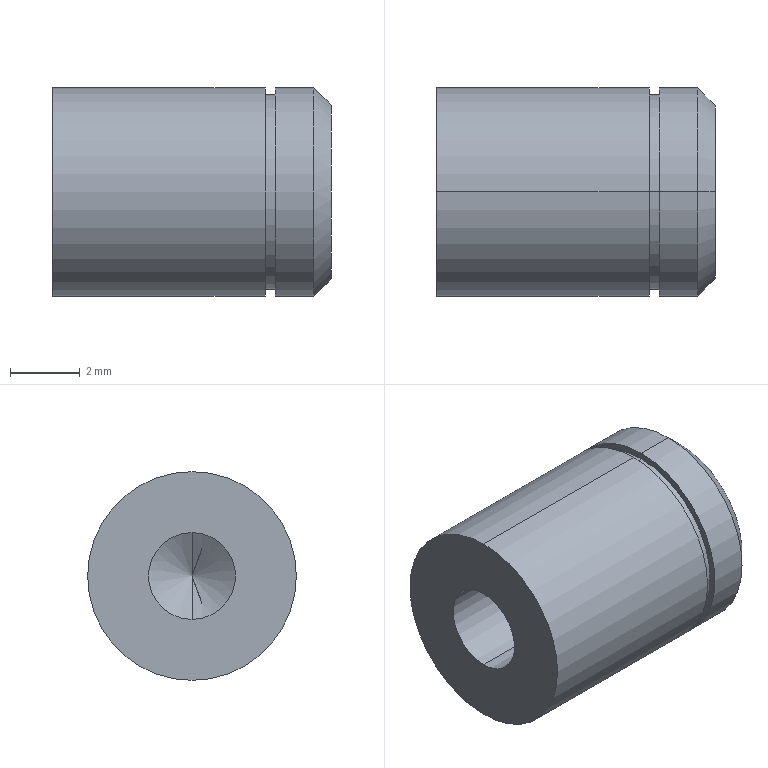Part | SolidWorks | features 3DProfileFeature 1, Chamfer 1, Extrusion 1, HoleWzd 1, RevCut 1 | 1 solid | 16 faces | box 8 x 6 x 6 mm | volume 189.74 mm3 | cylinder 8 | cone 4 | plane 4 | commonest cylinder face diameters 6 x4 2.5 x2 5.6 x2
STEP:
#1=CARTESIAN_POINT('',(7.5,0.,3.));
#2=VERTEX_POINT('',#1);
#3=CARTESIAN_POINT('',(7.5,0.,-3.));
#4=VERTEX_POINT('',#3);
#5=CARTESIAN_POINT('',(7.5,0.,0.));
#6=DIRECTION('',(-1.,0.,0.));
#7=DIRECTION('',(0.,0.,-1.));
#8=AXIS2_PLACEMENT_3D('',#5,#6,#7);
#9=CIRCLE('',#8,3.);
#10=EDGE_CURVE('',#2,#4,#9,.T.);
#11=ORIENTED_EDGE('',*,*,#10,.T.);
#12=CARTESIAN_POINT('',(6.4,0.,-3.));
#13=VERTEX_POINT('',#12);
#14=CARTESIAN_POINT('',(8.,0.,-3.));
#15=DIRECTION('',(-1.,0.,0.));
#16=VECTOR('',#15,1000.);
#17=LINE('',#14,#16);
#18=EDGE_CURVE('',#4,#13,#17,.T.);
#19=ORIENTED_EDGE('',*,*,#18,.T.);
#20=CARTESIAN_POINT('',(6.4,0.,3.));
#21=VERTEX_POINT('',#20);
#22=CARTESIAN_POINT('',(6.4,0.,0.));
#23=DIRECTION('',(-1.,0.,0.));
#24=DIRECTION('',(0.,0.,1.));
#25=AXIS2_PLACEMENT_3D('',#22,#23,#24);
#26=CIRCLE('',#25,3.);
#27=EDGE_CURVE('',#21,#13,#26,.T.);
#28=ORIENTED_EDGE('',*,*,#27,.F.);
#29=CARTESIAN_POINT('',(8.,0.,3.));
#30=DIRECTION('',(-1.,0.,0.));
#31=VECTOR('',#30,1000.);
#32=LINE('',#29,#31);
#33=EDGE_CURVE('',#2,#21,#32,.T.);
#34=ORIENTED_EDGE('',*,*,#33,.F.);
#35=EDGE_LOOP('',(#11,#19,#28,#34));
#36=FACE_OUTER_BOUND('',#35,.T.);
#37=CARTESIAN_POINT('',(8.,0.,0.));
#38=DIRECTION('',(-1.,0.,0.));
#39=DIRECTION('',(0.,0.,1.));
#40=AXIS2_PLACEMENT_3D('',#37,#38,#39);
#41=CYLINDRICAL_SURFACE('',#40,3.);
#42=ADVANCED_FACE('',(#36),#41,.T.);
#43=CARTESIAN_POINT('',(8.,0.,-2.5));
#44=VERTEX_POINT('',#43);
#45=CARTESIAN_POINT('',(8.,0.,2.5));
#46=VERTEX_POINT('',#45);
#47=CARTESIAN_POINT('',(8.,0.,0.));
#48=DIRECTION('',(1.,0.,0.));
#49=DIRECTION('',(0.,0.,-1.));
#50=AXIS2_PLACEMENT_3D('',#47,#48,#49);
#51=CIRCLE('',#50,2.5);
#52=EDGE_CURVE('',#44,#46,#51,.T.);
#53=ORIENTED_EDGE('',*,*,#52,.F.);
#54=CARTESIAN_POINT('',(8.,0.,-2.5));
#55=DIRECTION('',(-0.7071,0.,-0.7071));
#56=VECTOR('',#55,1000.);
#57=LINE('',#54,#56);
#58=EDGE_CURVE('',#44,#4,#57,.T.);
#59=ORIENTED_EDGE('',*,*,#58,.T.);
#60=ORIENTED_EDGE('',*,*,#10,.F.);
#61=CARTESIAN_POINT('',(8.,0.,2.5));
#62=DIRECTION('',(-0.7071,0.,0.7071));
#63=VECTOR('',#62,1000.);
#64=LINE('',#61,#63);
#65=EDGE_CURVE('',#46,#2,#64,.T.);
#66=ORIENTED_EDGE('',*,*,#65,.F.);
#67=EDGE_LOOP('',(#53,#59,#60,#66));
#68=FACE_OUTER_BOUND('',#67,.T.);
#69=CARTESIAN_POINT('',(8.,0.,0.));
#70=DIRECTION('',(-1.,0.,0.));
#71=DIRECTION('',(0.,0.,1.));
#72=AXIS2_PLACEMENT_3D('',#69,#70,#71);
#73=CONICAL_SURFACE('',#72,2.5,0.7854);
#74=ADVANCED_FACE('',(#68),#73,.T.);
#75=CARTESIAN_POINT('',(6.4,0.,2.8));
#76=VERTEX_POINT('',#75);
#77=CARTESIAN_POINT('',(6.4,0.,-2.8));
#78=VERTEX_POINT('',#77);
#79=CARTESIAN_POINT('',(6.4,0.,0.));
#80=DIRECTION('',(-1.,0.,0.));
#81=DIRECTION('',(0.,0.,1.));
#82=AXIS2_PLACEMENT_3D('',#79,#80,#81);
#83=CIRCLE('',#82,2.8);
#84=EDGE_CURVE('',#76,#78,#83,.T.);
#85=ORIENTED_EDGE('',*,*,#84,.T.);
#86=CARTESIAN_POINT('',(6.1,0.,-2.8));
#87=VERTEX_POINT('',#86);
#88=CARTESIAN_POINT('',(0.,0.,-2.8));
#89=DIRECTION('',(-1.,0.,0.));
#90=VECTOR('',#89,1000.);
#91=LINE('',#88,#90);
#92=EDGE_CURVE('',#78,#87,#91,.T.);
#93=ORIENTED_EDGE('',*,*,#92,.T.);
#94=CARTESIAN_POINT('',(6.1,0.,2.8));
#95=VERTEX_POINT('',#94);
#96=CARTESIAN_POINT('',(6.1,0.,0.));
#97=DIRECTION('',(-1.,0.,0.));
#98=DIRECTION('',(0.,0.,1.));
#99=AXIS2_PLACEMENT_3D('',#96,#97,#98);
#100=CIRCLE('',#99,2.8);
#101=EDGE_CURVE('',#95,#87,#100,.T.);
#102=ORIENTED_EDGE('',*,*,#101,.F.);
#103=CARTESIAN_POINT('',(0.,0.,2.8));
#104=DIRECTION('',(-1.,0.,0.));
#105=VECTOR('',#104,1000.);
#106=LINE('',#103,#105);
#107=EDGE_CURVE('',#76,#95,#106,.T.);
#108=ORIENTED_EDGE('',*,*,#107,.F.);
#109=EDGE_LOOP('',(#85,#93,#102,#108));
#110=FACE_OUTER_BOUND('',#109,.T.);
#111=CARTESIAN_POINT('',(0.,0.,0.));
#112=DIRECTION('',(-1.,0.,0.));
#113=DIRECTION('',(0.,0.,1.));
#114=AXIS2_PLACEMENT_3D('',#111,#112,#113);
#115=CYLINDRICAL_SURFACE('',#114,2.8);
#116=ADVANCED_FACE('',(#110),#115,.T.);
#117=CARTESIAN_POINT('',(6.5,0.,-1.25));
#118=VERTEX_POINT('',#117);
#119=CARTESIAN_POINT('',(6.5,0.,1.25));
#120=VERTEX_POINT('',#119);
#121=CARTESIAN_POINT('',(6.5,0.,0.));
#122=DIRECTION('',(-1.,0.,0.));
#123=DIRECTION('',(0.,0.,1.));
#124=AXIS2_PLACEMENT_3D('',#121,#122,#123);
#125=CIRCLE('',#124,1.25);
#126=EDGE_CURVE('',#118,#120,#125,.T.);
#127=ORIENTED_EDGE('',*,*,#126,.F.);
#128=CARTESIAN_POINT('',(0.,0.,-1.25));
#129=VERTEX_POINT('',#128);
#130=CARTESIAN_POINT('',(0.,0.,-1.25));
#131=DIRECTION('',(-1.,0.,0.));
#132=VECTOR('',#131,1000.);
#133=LINE('',#130,#132);
#134=EDGE_CURVE('',#118,#129,#133,.T.);
#135=ORIENTED_EDGE('',*,*,#134,.T.);
#136=CARTESIAN_POINT('',(0.,0.,1.25));
#137=VERTEX_POINT('',#136);
#138=CARTESIAN_POINT('',(0.,0.,0.));
#139=DIRECTION('',(-1.,0.,0.));
#140=DIRECTION('',(0.,0.,1.));
#141=AXIS2_PLACEMENT_3D('',#138,#139,#140);
#142=CIRCLE('',#141,1.25);
#143=EDGE_CURVE('',#129,#137,#142,.T.);
#144=ORIENTED_EDGE('',*,*,#143,.T.);
#145=CARTESIAN_POINT('',(0.,0.,1.25));
#146=DIRECTION('',(-1.,0.,0.));
#147=VECTOR('',#146,1000.);
#148=LINE('',#145,#147);
#149=EDGE_CURVE('',#120,#137,#148,.T.);
#150=ORIENTED_EDGE('',*,*,#149,.F.);
#151=EDGE_LOOP('',(#127,#135,#144,#150));
#152=FACE_OUTER_BOUND('',#151,.T.);
#153=CARTESIAN_POINT('',(0.,0.,0.));
#154=DIRECTION('',(-1.,0.,0.));
#155=DIRECTION('',(0.,0.,1.));
#156=AXIS2_PLACEMENT_3D('',#153,#154,#155);
#157=CYLINDRICAL_SURFACE('',#156,1.25);
#158=ADVANCED_FACE('',(#152),#157,.F.);
#159=CARTESIAN_POINT('',(7.251,0.,0.));
#160=VERTEX_POINT('',#159);
#161=CARTESIAN_POINT('',(6.5,0.,1.25));
#162=DIRECTION('',(-0.515,0.,0.8572));
#163=VECTOR('',#162,1000.);
#164=LINE('',#161,#163);
#165=EDGE_CURVE('',#160,#120,#164,.T.);
#166=ORIENTED_EDGE('',*,*,#165,.F.);
#167=CARTESIAN_POINT('',(6.5,0.,-1.25));
#168=DIRECTION('',(-0.515,0.,-0.8572));
#169=VECTOR('',#168,1000.);
#170=LINE('',#167,#169);
#171=EDGE_CURVE('',#160,#118,#170,.T.);
#172=ORIENTED_EDGE('',*,*,#171,.T.);
#173=ORIENTED_EDGE('',*,*,#126,.T.);
#174=EDGE_LOOP('',(#166,#172,#173));
#175=FACE_OUTER_BOUND('',#174,.T.);
#176=CARTESIAN_POINT('',(6.5,0.,0.));
#177=DIRECTION('',(-1.,0.,0.));
#178=DIRECTION('',(0.,0.,1.));
#179=AXIS2_PLACEMENT_3D('',#176,#177,#178);
#180=CONICAL_SURFACE('',#179,1.25,1.03);
#181=ADVANCED_FACE('',(#175),#180,.F.);
#182=CARTESIAN_POINT('',(6.1,0.,3.));
#183=VERTEX_POINT('',#182);
#184=CARTESIAN_POINT('',(6.1,0.,-3.));
#185=VERTEX_POINT('',#184);
#186=CARTESIAN_POINT('',(6.1,0.,0.));
#187=DIRECTION('',(-1.,0.,0.));
#188=DIRECTION('',(0.,0.,1.));
#189=AXIS2_PLACEMENT_3D('',#186,#187,#188);
#190=CIRCLE('',#189,3.);
#191=EDGE_CURVE('',#183,#185,#190,.T.);
#192=ORIENTED_EDGE('',*,*,#191,.T.);
#193=CARTESIAN_POINT('',(0.,0.,-3.));
#194=VERTEX_POINT('',#193);
#195=CARTESIAN_POINT('',(8.,0.,-3.));
#196=DIRECTION('',(-1.,0.,0.));
#197=VECTOR('',#196,1000.);
#198=LINE('',#195,#197);
#199=EDGE_CURVE('',#185,#194,#198,.T.);
#200=ORIENTED_EDGE('',*,*,#199,.T.);
#201=CARTESIAN_POINT('',(0.,0.,3.));
#202=VERTEX_POINT('',#201);
#203=CARTESIAN_POINT('',(0.,0.,0.));
#204=DIRECTION('',(1.,0.,0.));
#205=DIRECTION('',(0.,0.,-1.));
#206=AXIS2_PLACEMENT_3D('',#203,#204,#205);
#207=CIRCLE('',#206,3.);
#208=EDGE_CURVE('',#194,#202,#207,.T.);
#209=ORIENTED_EDGE('',*,*,#208,.T.);
#210=CARTESIAN_POINT('',(8.,0.,3.));
#211=DIRECTION('',(-1.,0.,0.));
#212=VECTOR('',#211,1000.);
#213=LINE('',#210,#212);
#214=EDGE_CURVE('',#183,#202,#213,.T.);
#215=ORIENTED_EDGE('',*,*,#214,.F.);
#216=EDGE_LOOP('',(#192,#200,#209,#215));
#217=FACE_OUTER_BOUND('',#216,.T.);
#218=CARTESIAN_POINT('',(8.,0.,0.));
#219=DIRECTION('',(-1.,0.,0.));
#220=DIRECTION('',(0.,0.,1.));
#221=AXIS2_PLACEMENT_3D('',#218,#219,#220);
#222=CYLINDRICAL_SURFACE('',#221,3.);
#223=ADVANCED_FACE('',(#217),#222,.T.);
#224=ORIENTED_EDGE('',*,*,#199,.F.);
#225=CARTESIAN_POINT('',(6.1,0.,0.));
#226=DIRECTION('',(-1.,0.,0.));
#227=DIRECTION('',(0.,0.,1.));
#228=AXIS2_PLACEMENT_3D('',#225,#226,#227);
#229=CIRCLE('',#228,3.);
#230=EDGE_CURVE('',#185,#183,#229,.T.);
#231=ORIENTED_EDGE('',*,*,#230,.T.);
#232=ORIENTED_EDGE('',*,*,#214,.T.);
#233=CARTESIAN_POINT('',(0.,0.,0.));
#234=DIRECTION('',(1.,0.,0.));
#235=DIRECTION('',(0.,0.,-1.));
#236=AXIS2_PLACEMENT_3D('',#233,#234,#235);
#237=CIRCLE('',#236,3.);
#238=EDGE_CURVE('',#202,#194,#237,.T.);
#239=ORIENTED_EDGE('',*,*,#238,.T.);
#240=EDGE_LOOP('',(#224,#231,#232,#239));
#241=FACE_OUTER_BOUND('',#240,.T.);
#242=CARTESIAN_POINT('',(8.,0.,0.));
#243=DIRECTION('',(-1.,0.,0.));
#244=DIRECTION('',(0.,0.,1.));
#245=AXIS2_PLACEMENT_3D('',#242,#243,#244);
#246=CYLINDRICAL_SURFACE('',#245,3.);
#247=ADVANCED_FACE('',(#241),#246,.T.);
#248=CARTESIAN_POINT('',(0.,0.,0.));
#249=DIRECTION('',(-1.,0.,0.));
#250=DIRECTION('',(0.,0.,1.));
#251=AXIS2_PLACEMENT_3D('',#248,#249,#250);
#252=CIRCLE('',#251,1.25);
#253=EDGE_CURVE('',#137,#129,#252,.T.);
#254=ORIENTED_EDGE('',*,*,#253,.F.);
#255=ORIENTED_EDGE('',*,*,#143,.F.);
#256=EDGE_LOOP('',(#254,#255));
#257=FACE_BOUND('',#256,.T.);
#258=ORIENTED_EDGE('',*,*,#238,.F.);
#259=ORIENTED_EDGE('',*,*,#208,.F.);
#260=EDGE_LOOP('',(#258,#259));
#261=FACE_OUTER_BOUND('',#260,.T.);
#262=CARTESIAN_POINT('',(0.,0.,0.));
#263=DIRECTION('',(1.,0.,0.));
#264=DIRECTION('',(0.,0.,-1.));
#265=AXIS2_PLACEMENT_3D('',#262,#263,#264);
#266=PLANE('',#265);
#267=ADVANCED_FACE('',(#257,#261),#266,.F.);
#268=ORIENTED_EDGE('',*,*,#171,.F.);
#269=ORIENTED_EDGE('',*,*,#165,.T.);
#270=CARTESIAN_POINT('',(6.5,0.,0.));
#271=DIRECTION('',(-1.,0.,0.));
#272=DIRECTION('',(0.,0.,1.));
#273=AXIS2_PLACEMENT_3D('',#270,#271,#272);
#274=CIRCLE('',#273,1.25);
#275=EDGE_CURVE('',#120,#118,#274,.T.);
#276=ORIENTED_EDGE('',*,*,#275,.T.);
#277=EDGE_LOOP('',(#268,#269,#276));
#278=FACE_OUTER_BOUND('',#277,.T.);
#279=CARTESIAN_POINT('',(6.5,0.,0.));
#280=DIRECTION('',(-1.,0.,0.));
#281=DIRECTION('',(0.,0.,1.));
#282=AXIS2_PLACEMENT_3D('',#279,#280,#281);
#283=CONICAL_SURFACE('',#282,1.25,1.03);
#284=ADVANCED_FACE('',(#278),#283,.F.);
#285=ORIENTED_EDGE('',*,*,#134,.F.);
#286=ORIENTED_EDGE('',*,*,#275,.F.);
#287=ORIENTED_EDGE('',*,*,#149,.T.);
#288=ORIENTED_EDGE('',*,*,#253,.T.);
#289=EDGE_LOOP('',(#285,#286,#287,#288));
#290=FACE_OUTER_BOUND('',#289,.T.);
#291=CARTESIAN_POINT('',(0.,0.,0.));
#292=DIRECTION('',(-1.,0.,0.));
#293=DIRECTION('',(0.,0.,1.));
#294=AXIS2_PLACEMENT_3D('',#291,#292,#293);
#295=CYLINDRICAL_SURFACE('',#294,1.25);
#296=ADVANCED_FACE('',(#290),#295,.F.);
#297=ORIENTED_EDGE('',*,*,#101,.T.);
#298=CARTESIAN_POINT('',(6.1,0.,0.));
#299=DIRECTION('',(-1.,0.,0.));
#300=DIRECTION('',(0.,0.,1.));
#301=AXIS2_PLACEMENT_3D('',#298,#299,#300);
#302=CIRCLE('',#301,2.8);
#303=EDGE_CURVE('',#87,#95,#302,.T.);
#304=ORIENTED_EDGE('',*,*,#303,.T.);
#305=EDGE_LOOP('',(#297,#304));
#306=FACE_BOUND('',#305,.T.);
#307=ORIENTED_EDGE('',*,*,#191,.F.);
#308=ORIENTED_EDGE('',*,*,#230,.F.);
#309=EDGE_LOOP('',(#307,#308));
#310=FACE_OUTER_BOUND('',#309,.T.);
#311=CARTESIAN_POINT('',(6.1,0.,-3.));
#312=DIRECTION('',(1.,0.,0.));
#313=DIRECTION('',(0.,0.,-1.));
#314=AXIS2_PLACEMENT_3D('',#311,#312,#313);
#315=PLANE('',#314);
#316=ADVANCED_FACE('',(#306,#310),#315,.T.);
#317=ORIENTED_EDGE('',*,*,#92,.F.);
#318=CARTESIAN_POINT('',(6.4,0.,0.));
#319=DIRECTION('',(-1.,0.,0.));
#320=DIRECTION('',(0.,0.,1.));
#321=AXIS2_PLACEMENT_3D('',#318,#319,#320);
#322=CIRCLE('',#321,2.8);
#323=EDGE_CURVE('',#78,#76,#322,.T.);
#324=ORIENTED_EDGE('',*,*,#323,.T.);
#325=ORIENTED_EDGE('',*,*,#107,.T.);
#326=ORIENTED_EDGE('',*,*,#303,.F.);
#327=EDGE_LOOP('',(#317,#324,#325,#326));
#328=FACE_OUTER_BOUND('',#327,.T.);
#329=CARTESIAN_POINT('',(0.,0.,0.));
#330=DIRECTION('',(-1.,0.,0.));
#331=DIRECTION('',(0.,0.,1.));
#332=AXIS2_PLACEMENT_3D('',#329,#330,#331);
#333=CYLINDRICAL_SURFACE('',#332,2.8);
#334=ADVANCED_FACE('',(#328),#333,.T.);
#335=ORIENTED_EDGE('',*,*,#27,.T.);
#336=CARTESIAN_POINT('',(6.4,0.,0.));
#337=DIRECTION('',(-1.,0.,0.));
#338=DIRECTION('',(0.,0.,1.));
#339=AXIS2_PLACEMENT_3D('',#336,#337,#338);
#340=CIRCLE('',#339,3.);
#341=EDGE_CURVE('',#13,#21,#340,.T.);
#342=ORIENTED_EDGE('',*,*,#341,.T.);
#343=EDGE_LOOP('',(#335,#342));
#344=FACE_OUTER_BOUND('',#343,.T.);
#345=ORIENTED_EDGE('',*,*,#84,.F.);
#346=ORIENTED_EDGE('',*,*,#323,.F.);
#347=EDGE_LOOP('',(#345,#346));
#348=FACE_BOUND('',#347,.T.);
#349=CARTESIAN_POINT('',(6.4,0.,-3.));
#350=DIRECTION('',(-1.,0.,0.));
#351=DIRECTION('',(0.,0.,1.));
#352=AXIS2_PLACEMENT_3D('',#349,#350,#351);
#353=PLANE('',#352);
#354=ADVANCED_FACE('',(#344,#348),#353,.T.);
#355=CARTESIAN_POINT('',(8.,0.,0.));
#356=DIRECTION('',(1.,0.,0.));
#357=DIRECTION('',(0.,0.,-1.));
#358=AXIS2_PLACEMENT_3D('',#355,#356,#357);
#359=CIRCLE('',#358,2.5);
#360=EDGE_CURVE('',#46,#44,#359,.T.);
#361=ORIENTED_EDGE('',*,*,#360,.T.);
#362=ORIENTED_EDGE('',*,*,#52,.T.);
#363=EDGE_LOOP('',(#361,#362));
#364=FACE_OUTER_BOUND('',#363,.T.);
#365=CARTESIAN_POINT('',(8.,0.,0.));
#366=DIRECTION('',(1.,0.,0.));
#367=DIRECTION('',(0.,0.,-1.));
#368=AXIS2_PLACEMENT_3D('',#365,#366,#367);
#369=PLANE('',#368);
#370=ADVANCED_FACE('',(#364),#369,.T.);
#371=ORIENTED_EDGE('',*,*,#58,.F.);
#372=ORIENTED_EDGE('',*,*,#360,.F.);
#373=ORIENTED_EDGE('',*,*,#65,.T.);
#374=CARTESIAN_POINT('',(7.5,0.,0.));
#375=DIRECTION('',(-1.,0.,0.));
#376=DIRECTION('',(0.,0.,-1.));
#377=AXIS2_PLACEMENT_3D('',#374,#375,#376);
#378=CIRCLE('',#377,3.);
#379=EDGE_CURVE('',#4,#2,#378,.T.);
#380=ORIENTED_EDGE('',*,*,#379,.F.);
#381=EDGE_LOOP('',(#371,#372,#373,#380));
#382=FACE_OUTER_BOUND('',#381,.T.);
#383=CARTESIAN_POINT('',(8.,0.,0.));
#384=DIRECTION('',(-1.,0.,0.));
#385=DIRECTION('',(0.,0.,1.));
#386=AXIS2_PLACEMENT_3D('',#383,#384,#385);
#387=CONICAL_SURFACE('',#386,2.5,0.7854);
#388=ADVANCED_FACE('',(#382),#387,.T.);
#389=ORIENTED_EDGE('',*,*,#18,.F.);
#390=ORIENTED_EDGE('',*,*,#379,.T.);
#391=ORIENTED_EDGE('',*,*,#33,.T.);
#392=ORIENTED_EDGE('',*,*,#341,.F.);
#393=EDGE_LOOP('',(#389,#390,#391,#392));
#394=FACE_OUTER_BOUND('',#393,.T.);
#395=CARTESIAN_POINT('',(8.,0.,0.));
#396=DIRECTION('',(-1.,0.,0.));
#397=DIRECTION('',(0.,0.,1.));
#398=AXIS2_PLACEMENT_3D('',#395,#396,#397);
#399=CYLINDRICAL_SURFACE('',#398,3.);
#400=ADVANCED_FACE('',(#394),#399,.T.);
#401=CLOSED_SHELL('',(#42,#74,#116,#158,#181,#223,#247,#267,#284,#296,#316,#334,#354,#370,#388,#400));
#402=MANIFOLD_SOLID_BREP('',#401);
#403=CARTESIAN_POINT('',(0.,0.,0.));
#404=DIRECTION('',(0.,0.,1.));
#405=DIRECTION('',(1.,0.,0.));
#406=AXIS2_PLACEMENT_3D('',#403,#404,#405);
#407=(LENGTH_UNIT()NAMED_UNIT(*)SI_UNIT(.MILLI.,.METRE.));
#408=UNCERTAINTY_MEASURE_WITH_UNIT(LENGTH_MEASURE(0.00001),#407,'','');
#409=(NAMED_UNIT(*)PLANE_ANGLE_UNIT()SI_UNIT($,.RADIAN.));
#410=(NAMED_UNIT(*)SI_UNIT($,.STERADIAN.)SOLID_ANGLE_UNIT());
#411=(GEOMETRIC_REPRESENTATION_CONTEXT(3)GLOBAL_UNCERTAINTY_ASSIGNED_CONTEXT((#408))GLOBAL_UNIT_ASSIGNED_CONTEXT((#407,#409,#410))REPRESENTATION_CONTEXT('',''));
#412=ADVANCED_BREP_SHAPE_REPRESENTATION('',(#402,#406),#411);